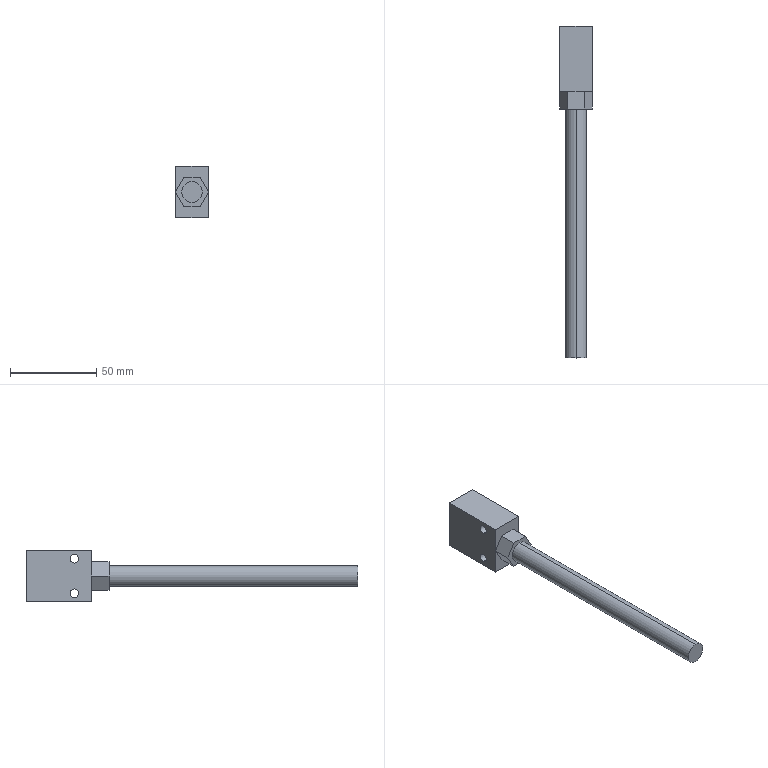Part | STEP file | Blowing port | 1 solid | 25 faces | box 19 x 192 x 30 mm | volume 38106 mm3 | plane 15 | cylinder 8 | cone 2 | commonest cylinder face diameters 5 x4 8.5 x2 12 x2
STEP:
#1=CARTESIAN_POINT('',(0.,-173.,6.));
#2=VERTEX_POINT('',#1);
#3=CARTESIAN_POINT('',(0.,-173.,-6.));
#4=VERTEX_POINT('',#3);
#5=CARTESIAN_POINT('',(0.,-173.,0.));
#6=DIRECTION('',(0.,1.,0.));
#7=DIRECTION('',(0.,0.,1.));
#8=AXIS2_PLACEMENT_3D('',#5,#6,#7);
#9=CIRCLE('',#8,6.);
#10=EDGE_CURVE('',#2,#4,#9,.T.);
#11=ORIENTED_EDGE('',*,*,#10,.T.);
#12=CARTESIAN_POINT('',(0.,-29.,-6.));
#13=VERTEX_POINT('',#12);
#14=CARTESIAN_POINT('',(0.,-173.,-6.));
#15=DIRECTION('',(0.,1.,0.));
#16=VECTOR('',#15,1000.);
#17=LINE('',#14,#16);
#18=EDGE_CURVE('',#4,#13,#17,.T.);
#19=ORIENTED_EDGE('',*,*,#18,.T.);
#20=CARTESIAN_POINT('',(0.,-29.,6.));
#21=VERTEX_POINT('',#20);
#22=CARTESIAN_POINT('',(0.,-29.,0.));
#23=DIRECTION('',(0.,-1.,0.));
#24=DIRECTION('',(0.,0.,1.));
#25=AXIS2_PLACEMENT_3D('',#22,#23,#24);
#26=CIRCLE('',#25,6.);
#27=EDGE_CURVE('',#13,#21,#26,.T.);
#28=ORIENTED_EDGE('',*,*,#27,.T.);
#29=CARTESIAN_POINT('',(0.,-173.,6.));
#30=DIRECTION('',(0.,1.,0.));
#31=VECTOR('',#30,1000.);
#32=LINE('',#29,#31);
#33=EDGE_CURVE('',#2,#21,#32,.T.);
#34=ORIENTED_EDGE('',*,*,#33,.F.);
#35=EDGE_LOOP('',(#11,#19,#28,#34));
#36=FACE_OUTER_BOUND('',#35,.T.);
#37=CARTESIAN_POINT('',(0.,-173.,0.));
#38=DIRECTION('',(0.,1.,0.));
#39=DIRECTION('',(0.,0.,1.));
#40=AXIS2_PLACEMENT_3D('',#37,#38,#39);
#41=CYLINDRICAL_SURFACE('',#40,6.);
#42=ADVANCED_FACE('',(#36),#41,.T.);
#43=CARTESIAN_POINT('',(9.5,-9.,-7.5));
#44=VERTEX_POINT('',#43);
#45=CARTESIAN_POINT('',(9.5,-9.,-12.5));
#46=VERTEX_POINT('',#45);
#47=CARTESIAN_POINT('',(9.5,-9.,-10.));
#48=DIRECTION('',(1.,0.,0.));
#49=DIRECTION('',(0.,0.,1.));
#50=AXIS2_PLACEMENT_3D('',#47,#48,#49);
#51=CIRCLE('',#50,2.5);
#52=EDGE_CURVE('',#44,#46,#51,.T.);
#53=ORIENTED_EDGE('',*,*,#52,.T.);
#54=CARTESIAN_POINT('',(-9.5,-9.,-12.5));
#55=VERTEX_POINT('',#54);
#56=CARTESIAN_POINT('',(9.5,-9.,-12.5));
#57=DIRECTION('',(-1.,0.,0.));
#58=VECTOR('',#57,1000.);
#59=LINE('',#56,#58);
#60=EDGE_CURVE('',#46,#55,#59,.T.);
#61=ORIENTED_EDGE('',*,*,#60,.T.);
#62=CARTESIAN_POINT('',(-9.5,-9.,-7.5));
#63=VERTEX_POINT('',#62);
#64=CARTESIAN_POINT('',(-9.5,-9.,-10.));
#65=DIRECTION('',(1.,0.,0.));
#66=DIRECTION('',(0.,0.,1.));
#67=AXIS2_PLACEMENT_3D('',#64,#65,#66);
#68=CIRCLE('',#67,2.5);
#69=EDGE_CURVE('',#63,#55,#68,.T.);
#70=ORIENTED_EDGE('',*,*,#69,.F.);
#71=CARTESIAN_POINT('',(9.5,-9.,-7.5));
#72=DIRECTION('',(-1.,0.,0.));
#73=VECTOR('',#72,1000.);
#74=LINE('',#71,#73);
#75=EDGE_CURVE('',#44,#63,#74,.T.);
#76=ORIENTED_EDGE('',*,*,#75,.F.);
#77=EDGE_LOOP('',(#53,#61,#70,#76));
#78=FACE_OUTER_BOUND('',#77,.T.);
#79=CARTESIAN_POINT('',(9.5,-9.,-10.));
#80=DIRECTION('',(-1.,0.,0.));
#81=DIRECTION('',(0.,0.,1.));
#82=AXIS2_PLACEMENT_3D('',#79,#80,#81);
#83=CYLINDRICAL_SURFACE('',#82,2.5);
#84=ADVANCED_FACE('',(#78),#83,.F.);
#85=CARTESIAN_POINT('',(9.5,-9.,12.5));
#86=VERTEX_POINT('',#85);
#87=CARTESIAN_POINT('',(9.5,-9.,7.5));
#88=VERTEX_POINT('',#87);
#89=CARTESIAN_POINT('',(9.5,-9.,10.));
#90=DIRECTION('',(1.,0.,0.));
#91=DIRECTION('',(0.,0.,1.));
#92=AXIS2_PLACEMENT_3D('',#89,#90,#91);
#93=CIRCLE('',#92,2.5);
#94=EDGE_CURVE('',#86,#88,#93,.T.);
#95=ORIENTED_EDGE('',*,*,#94,.T.);
#96=CARTESIAN_POINT('',(-9.5,-9.,7.5));
#97=VERTEX_POINT('',#96);
#98=CARTESIAN_POINT('',(9.5,-9.,7.5));
#99=DIRECTION('',(-1.,0.,0.));
#100=VECTOR('',#99,1000.);
#101=LINE('',#98,#100);
#102=EDGE_CURVE('',#88,#97,#101,.T.);
#103=ORIENTED_EDGE('',*,*,#102,.T.);
#104=CARTESIAN_POINT('',(-9.5,-9.,12.5));
#105=VERTEX_POINT('',#104);
#106=CARTESIAN_POINT('',(-9.5,-9.,10.));
#107=DIRECTION('',(1.,0.,0.));
#108=DIRECTION('',(0.,0.,1.));
#109=AXIS2_PLACEMENT_3D('',#106,#107,#108);
#110=CIRCLE('',#109,2.5);
#111=EDGE_CURVE('',#105,#97,#110,.T.);
#112=ORIENTED_EDGE('',*,*,#111,.F.);
#113=CARTESIAN_POINT('',(9.5,-9.,12.5));
#114=DIRECTION('',(-1.,0.,0.));
#115=VECTOR('',#114,1000.);
#116=LINE('',#113,#115);
#117=EDGE_CURVE('',#86,#105,#116,.T.);
#118=ORIENTED_EDGE('',*,*,#117,.F.);
#119=EDGE_LOOP('',(#95,#103,#112,#118));
#120=FACE_OUTER_BOUND('',#119,.T.);
#121=CARTESIAN_POINT('',(9.5,-9.,10.));
#122=DIRECTION('',(-1.,0.,0.));
#123=DIRECTION('',(0.,0.,1.));
#124=AXIS2_PLACEMENT_3D('',#121,#122,#123);
#125=CYLINDRICAL_SURFACE('',#124,2.5);
#126=ADVANCED_FACE('',(#120),#125,.F.);
#127=CARTESIAN_POINT('',(4.25,12.609,9.5));
#128=VERTEX_POINT('',#127);
#129=CARTESIAN_POINT('',(-4.25,12.609,9.5));
#130=VERTEX_POINT('',#129);
#131=CARTESIAN_POINT('',(0.,12.609,9.5));
#132=DIRECTION('',(0.,0.,-1.));
#133=DIRECTION('',(-1.,0.,0.));
#134=AXIS2_PLACEMENT_3D('',#131,#132,#133);
#135=CIRCLE('',#134,4.25);
#136=EDGE_CURVE('',#128,#130,#135,.T.);
#137=ORIENTED_EDGE('',*,*,#136,.F.);
#138=CARTESIAN_POINT('',(4.25,12.609,-15.));
#139=VERTEX_POINT('',#138);
#140=CARTESIAN_POINT('',(4.25,12.609,-15.));
#141=DIRECTION('',(0.,0.,-1.));
#142=VECTOR('',#141,1000.);
#143=LINE('',#140,#142);
#144=EDGE_CURVE('',#128,#139,#143,.T.);
#145=ORIENTED_EDGE('',*,*,#144,.T.);
#146=CARTESIAN_POINT('',(-4.25,12.609,-15.));
#147=VERTEX_POINT('',#146);
#148=CARTESIAN_POINT('',(0.,12.609,-15.));
#149=DIRECTION('',(0.,0.,-1.));
#150=DIRECTION('',(-1.,0.,0.));
#151=AXIS2_PLACEMENT_3D('',#148,#149,#150);
#152=CIRCLE('',#151,4.25);
#153=EDGE_CURVE('',#139,#147,#152,.T.);
#154=ORIENTED_EDGE('',*,*,#153,.T.);
#155=CARTESIAN_POINT('',(-4.25,12.609,-15.));
#156=DIRECTION('',(0.,0.,-1.));
#157=VECTOR('',#156,1000.);
#158=LINE('',#155,#157);
#159=EDGE_CURVE('',#130,#147,#158,.T.);
#160=ORIENTED_EDGE('',*,*,#159,.F.);
#161=EDGE_LOOP('',(#137,#145,#154,#160));
#162=FACE_OUTER_BOUND('',#161,.T.);
#163=CARTESIAN_POINT('',(0.,12.609,-15.));
#164=DIRECTION('',(0.,0.,-1.));
#165=DIRECTION('',(-1.,0.,0.));
#166=AXIS2_PLACEMENT_3D('',#163,#164,#165);
#167=CYLINDRICAL_SURFACE('',#166,4.25);
#168=ADVANCED_FACE('',(#162),#167,.F.);
#169=CARTESIAN_POINT('',(0.,12.609,12.054));
#170=VERTEX_POINT('',#169);
#171=CARTESIAN_POINT('',(-4.25,12.609,9.5));
#172=DIRECTION('',(-0.8572,0.,-0.515));
#173=VECTOR('',#172,1000.);
#174=LINE('',#171,#173);
#175=EDGE_CURVE('',#170,#130,#174,.T.);
#176=ORIENTED_EDGE('',*,*,#175,.F.);
#177=CARTESIAN_POINT('',(4.25,12.609,9.5));
#178=DIRECTION('',(0.8572,0.,-0.515));
#179=VECTOR('',#178,1000.);
#180=LINE('',#177,#179);
#181=EDGE_CURVE('',#170,#128,#180,.T.);
#182=ORIENTED_EDGE('',*,*,#181,.T.);
#183=ORIENTED_EDGE('',*,*,#136,.T.);
#184=EDGE_LOOP('',(#176,#182,#183));
#185=FACE_OUTER_BOUND('',#184,.T.);
#186=CARTESIAN_POINT('',(0.,12.609,9.5));
#187=DIRECTION('',(0.,0.,-1.));
#188=DIRECTION('',(-1.,0.,0.));
#189=AXIS2_PLACEMENT_3D('',#186,#187,#188);
#190=CONICAL_SURFACE('',#189,4.25,1.03);
#191=ADVANCED_FACE('',(#185),#190,.F.);
#192=ORIENTED_EDGE('',*,*,#18,.F.);
#193=CARTESIAN_POINT('',(0.,-173.,0.));
#194=DIRECTION('',(0.,1.,0.));
#195=DIRECTION('',(0.,0.,1.));
#196=AXIS2_PLACEMENT_3D('',#193,#194,#195);
#197=CIRCLE('',#196,6.);
#198=EDGE_CURVE('',#4,#2,#197,.T.);
#199=ORIENTED_EDGE('',*,*,#198,.T.);
#200=ORIENTED_EDGE('',*,*,#33,.T.);
#201=CARTESIAN_POINT('',(0.,-29.,0.));
#202=DIRECTION('',(0.,-1.,0.));
#203=DIRECTION('',(0.,0.,1.));
#204=AXIS2_PLACEMENT_3D('',#201,#202,#203);
#205=CIRCLE('',#204,6.);
#206=EDGE_CURVE('',#21,#13,#205,.T.);
#207=ORIENTED_EDGE('',*,*,#206,.T.);
#208=EDGE_LOOP('',(#192,#199,#200,#207));
#209=FACE_OUTER_BOUND('',#208,.T.);
#210=CARTESIAN_POINT('',(0.,-173.,0.));
#211=DIRECTION('',(0.,1.,0.));
#212=DIRECTION('',(0.,0.,1.));
#213=AXIS2_PLACEMENT_3D('',#210,#211,#212);
#214=CYLINDRICAL_SURFACE('',#213,6.);
#215=ADVANCED_FACE('',(#209),#214,.T.);
#216=CARTESIAN_POINT('',(-9.5,-29.,0.));
#217=VERTEX_POINT('',#216);
#218=CARTESIAN_POINT('',(-4.75,-29.,-8.227));
#219=VERTEX_POINT('',#218);
#220=CARTESIAN_POINT('',(-9.5,-29.,0.));
#221=DIRECTION('',(0.5,0.,-0.866));
#222=VECTOR('',#221,1000.);
#223=LINE('',#220,#222);
#224=EDGE_CURVE('',#217,#219,#223,.T.);
#225=ORIENTED_EDGE('',*,*,#224,.T.);
#226=CARTESIAN_POINT('',(4.75,-29.,-8.227));
#227=VERTEX_POINT('',#226);
#228=CARTESIAN_POINT('',(0.,-29.,-8.227));
#229=DIRECTION('',(1.,0.,0.));
#230=VECTOR('',#229,1000.);
#231=LINE('',#228,#230);
#232=EDGE_CURVE('',#219,#227,#231,.T.);
#233=ORIENTED_EDGE('',*,*,#232,.T.);
#234=CARTESIAN_POINT('',(9.5,-29.,0.));
#235=VERTEX_POINT('',#234);
#236=CARTESIAN_POINT('',(4.75,-29.,-8.227));
#237=DIRECTION('',(0.5,0.,0.866));
#238=VECTOR('',#237,1000.);
#239=LINE('',#236,#238);
#240=EDGE_CURVE('',#227,#235,#239,.T.);
#241=ORIENTED_EDGE('',*,*,#240,.T.);
#242=CARTESIAN_POINT('',(4.75,-29.,8.227));
#243=VERTEX_POINT('',#242);
#244=CARTESIAN_POINT('',(9.5,-29.,0.));
#245=DIRECTION('',(-0.5,0.,0.866));
#246=VECTOR('',#245,1000.);
#247=LINE('',#244,#246);
#248=EDGE_CURVE('',#235,#243,#247,.T.);
#249=ORIENTED_EDGE('',*,*,#248,.T.);
#250=CARTESIAN_POINT('',(-4.75,-29.,8.227));
#251=VERTEX_POINT('',#250);
#252=CARTESIAN_POINT('',(0.,-29.,8.227));
#253=DIRECTION('',(-1.,0.,0.));
#254=VECTOR('',#253,1000.);
#255=LINE('',#252,#254);
#256=EDGE_CURVE('',#243,#251,#255,.T.);
#257=ORIENTED_EDGE('',*,*,#256,.T.);
#258=CARTESIAN_POINT('',(-4.75,-29.,8.227));
#259=DIRECTION('',(-0.5,0.,-0.866));
#260=VECTOR('',#259,1000.);
#261=LINE('',#258,#260);
#262=EDGE_CURVE('',#251,#217,#261,.T.);
#263=ORIENTED_EDGE('',*,*,#262,.T.);
#264=EDGE_LOOP('',(#225,#233,#241,#249,#257,#263));
#265=FACE_OUTER_BOUND('',#264,.T.);
#266=ORIENTED_EDGE('',*,*,#206,.F.);
#267=ORIENTED_EDGE('',*,*,#27,.F.);
#268=EDGE_LOOP('',(#266,#267));
#269=FACE_BOUND('',#268,.T.);
#270=CARTESIAN_POINT('',(0.,-29.,0.));
#271=DIRECTION('',(0.,-1.,0.));
#272=DIRECTION('',(0.,0.,-1.));
#273=AXIS2_PLACEMENT_3D('',#270,#271,#272);
#274=PLANE('',#273);
#275=ADVANCED_FACE('',(#265,#269),#274,.T.);
#276=ORIENTED_EDGE('',*,*,#10,.F.);
#277=ORIENTED_EDGE('',*,*,#198,.F.);
#278=EDGE_LOOP('',(#276,#277));
#279=FACE_OUTER_BOUND('',#278,.T.);
#280=CARTESIAN_POINT('',(0.,-173.,0.));
#281=DIRECTION('',(0.,-1.,0.));
#282=DIRECTION('',(0.,0.,-1.));
#283=AXIS2_PLACEMENT_3D('',#280,#281,#282);
#284=PLANE('',#283);
#285=ADVANCED_FACE('',(#279),#284,.T.);
#286=CARTESIAN_POINT('',(4.75,-19.,-8.227));
#287=VERTEX_POINT('',#286);
#288=CARTESIAN_POINT('',(4.75,-29.,-8.227));
#289=DIRECTION('',(0.,1.,0.));
#290=VECTOR('',#289,1000.);
#291=LINE('',#288,#290);
#292=EDGE_CURVE('',#227,#287,#291,.T.);
#293=ORIENTED_EDGE('',*,*,#292,.F.);
#294=ORIENTED_EDGE('',*,*,#232,.F.);
#295=CARTESIAN_POINT('',(-4.75,-19.,-8.227));
#296=VERTEX_POINT('',#295);
#297=CARTESIAN_POINT('',(-4.75,-29.,-8.227));
#298=DIRECTION('',(0.,-1.,0.));
#299=VECTOR('',#298,1000.);
#300=LINE('',#297,#299);
#301=EDGE_CURVE('',#296,#219,#300,.T.);
#302=ORIENTED_EDGE('',*,*,#301,.F.);
#303=CARTESIAN_POINT('',(-4.75,-19.,-8.227));
#304=DIRECTION('',(-1.,0.,0.));
#305=VECTOR('',#304,1000.);
#306=LINE('',#303,#305);
#307=EDGE_CURVE('',#287,#296,#306,.T.);
#308=ORIENTED_EDGE('',*,*,#307,.F.);
#309=EDGE_LOOP('',(#293,#294,#302,#308));
#310=FACE_OUTER_BOUND('',#309,.T.);
#311=CARTESIAN_POINT('',(-4.75,-29.,-8.227));
#312=DIRECTION('',(0.,0.,1.));
#313=DIRECTION('',(1.,0.,0.));
#314=AXIS2_PLACEMENT_3D('',#311,#312,#313);
#315=PLANE('',#314);
#316=ADVANCED_FACE('',(#310),#315,.F.);
#317=ORIENTED_EDGE('',*,*,#301,.T.);
#318=ORIENTED_EDGE('',*,*,#224,.F.);
#319=CARTESIAN_POINT('',(-9.5,-19.,0.));
#320=VERTEX_POINT('',#319);
#321=CARTESIAN_POINT('',(-9.5,-29.,0.));
#322=DIRECTION('',(0.,-1.,0.));
#323=VECTOR('',#322,1000.);
#324=LINE('',#321,#323);
#325=EDGE_CURVE('',#320,#217,#324,.T.);
#326=ORIENTED_EDGE('',*,*,#325,.F.);
#327=CARTESIAN_POINT('',(-9.5,-19.,0.));
#328=DIRECTION('',(-0.5,0.,0.866));
#329=VECTOR('',#328,1000.);
#330=LINE('',#327,#329);
#331=EDGE_CURVE('',#296,#320,#330,.T.);
#332=ORIENTED_EDGE('',*,*,#331,.F.);
#333=EDGE_LOOP('',(#317,#318,#326,#332));
#334=FACE_OUTER_BOUND('',#333,.T.);
#335=CARTESIAN_POINT('',(-9.5,-29.,0.));
#336=DIRECTION('',(0.866,0.,0.5));
#337=DIRECTION('',(0.5,0.,-0.866));
#338=AXIS2_PLACEMENT_3D('',#335,#336,#337);
#339=PLANE('',#338);
#340=ADVANCED_FACE('',(#334),#339,.F.);
#341=ORIENTED_EDGE('',*,*,#325,.T.);
#342=ORIENTED_EDGE('',*,*,#262,.F.);
#343=CARTESIAN_POINT('',(-4.75,-19.,8.227));
#344=VERTEX_POINT('',#343);
#345=CARTESIAN_POINT('',(-4.75,-29.,8.227));
#346=DIRECTION('',(0.,-1.,0.));
#347=VECTOR('',#346,1000.);
#348=LINE('',#345,#347);
#349=EDGE_CURVE('',#344,#251,#348,.T.);
#350=ORIENTED_EDGE('',*,*,#349,.F.);
#351=CARTESIAN_POINT('',(-4.75,-19.,8.227));
#352=DIRECTION('',(0.5,0.,0.866));
#353=VECTOR('',#352,1000.);
#354=LINE('',#351,#353);
#355=EDGE_CURVE('',#320,#344,#354,.T.);
#356=ORIENTED_EDGE('',*,*,#355,.F.);
#357=EDGE_LOOP('',(#341,#342,#350,#356));
#358=FACE_OUTER_BOUND('',#357,.T.);
#359=CARTESIAN_POINT('',(-4.75,-29.,8.227));
#360=DIRECTION('',(0.866,0.,-0.5));
#361=DIRECTION('',(-0.5,0.,-0.866));
#362=AXIS2_PLACEMENT_3D('',#359,#360,#361);
#363=PLANE('',#362);
#364=ADVANCED_FACE('',(#358),#363,.F.);
#365=ORIENTED_EDGE('',*,*,#349,.T.);
#366=ORIENTED_EDGE('',*,*,#256,.F.);
#367=CARTESIAN_POINT('',(4.75,-19.,8.227));
#368=VERTEX_POINT('',#367);
#369=CARTESIAN_POINT('',(4.75,-29.,8.227));
#370=DIRECTION('',(0.,-1.,0.));
#371=VECTOR('',#370,1000.);
#372=LINE('',#369,#371);
#373=EDGE_CURVE('',#368,#243,#372,.T.);
#374=ORIENTED_EDGE('',*,*,#373,.F.);
#375=CARTESIAN_POINT('',(4.75,-19.,8.227));
#376=DIRECTION('',(1.,0.,0.));
#377=VECTOR('',#376,1000.);
#378=LINE('',#375,#377);
#379=EDGE_CURVE('',#344,#368,#378,.T.);
#380=ORIENTED_EDGE('',*,*,#379,.F.);
#381=EDGE_LOOP('',(#365,#366,#374,#380));
#382=FACE_OUTER_BOUND('',#381,.T.);
#383=CARTESIAN_POINT('',(4.75,-29.,8.227));
#384=DIRECTION('',(0.,0.,-1.));
#385=DIRECTION('',(-1.,0.,0.));
#386=AXIS2_PLACEMENT_3D('',#383,#384,#385);
#387=PLANE('',#386);
#388=ADVANCED_FACE('',(#382),#387,.F.);
#389=ORIENTED_EDGE('',*,*,#373,.T.);
#390=ORIENTED_EDGE('',*,*,#248,.F.);
#391=CARTESIAN_POINT('',(9.5,-19.,0.));
#392=VERTEX_POINT('',#391);
#393=CARTESIAN_POINT('',(9.5,-29.,0.));
#394=DIRECTION('',(0.,-1.,0.));
#395=VECTOR('',#394,1000.);
#396=LINE('',#393,#395);
#397=EDGE_CURVE('',#392,#235,#396,.T.);
#398=ORIENTED_EDGE('',*,*,#397,.F.);
#399=CARTESIAN_POINT('',(9.5,-19.,0.));
#400=DIRECTION('',(0.5,0.,-0.866));
#401=VECTOR('',#400,1000.);
#402=LINE('',#399,#401);
#403=EDGE_CURVE('',#368,#392,#402,.T.);
#404=ORIENTED_EDGE('',*,*,#403,.F.);
#405=EDGE_LOOP('',(#389,#390,#398,#404));
#406=FACE_OUTER_BOUND('',#405,.T.);
#407=CARTESIAN_POINT('',(9.5,-29.,0.));
#408=DIRECTION('',(-0.866,0.,-0.5));
#409=DIRECTION('',(-0.5,0.,0.866));
#410=AXIS2_PLACEMENT_3D('',#407,#408,#409);
#411=PLANE('',#410);
#412=ADVANCED_FACE('',(#406),#411,.F.);
#413=ORIENTED_EDGE('',*,*,#397,.T.);
#414=ORIENTED_EDGE('',*,*,#240,.F.);
#415=ORIENTED_EDGE('',*,*,#292,.T.);
#416=CARTESIAN_POINT('',(4.75,-19.,-8.227));
#417=DIRECTION('',(-0.5,0.,-0.866));
#418=VECTOR('',#417,1000.);
#419=LINE('',#416,#418);
#420=EDGE_CURVE('',#392,#287,#419,.T.);
#421=ORIENTED_EDGE('',*,*,#420,.F.);
#422=EDGE_LOOP('',(#413,#414,#415,#421));
#423=FACE_OUTER_BOUND('',#422,.T.);
#424=CARTESIAN_POINT('',(4.75,-29.,-8.227));
#425=DIRECTION('',(-0.866,0.,0.5));
#426=DIRECTION('',(0.5,0.,0.866));
#427=AXIS2_PLACEMENT_3D('',#424,#425,#426);
#428=PLANE('',#427);
#429=ADVANCED_FACE('',(#423),#428,.F.);
#430=ORIENTED_EDGE('',*,*,#307,.T.);
#431=ORIENTED_EDGE('',*,*,#331,.T.);
#432=CARTESIAN_POINT('',(-9.5,-19.,-15.));
#433=VERTEX_POINT('',#432);
#434=CARTESIAN_POINT('',(-9.5,-19.,15.));
#435=DIRECTION('',(0.,0.,1.));
#436=VECTOR('',#435,1000.);
#437=LINE('',#434,#436);
#438=EDGE_CURVE('',#433,#320,#437,.T.);
#439=ORIENTED_EDGE('',*,*,#438,.F.);
#440=CARTESIAN_POINT('',(9.5,-19.,-15.));
#441=VERTEX_POINT('',#440);
#442=CARTESIAN_POINT('',(9.5,-19.,-15.));
#443=DIRECTION('',(-1.,0.,0.));
#444=VECTOR('',#443,1000.);
#445=LINE('',#442,#444);
#446=EDGE_CURVE('',#441,#433,#445,.T.);
#447=ORIENTED_EDGE('',*,*,#446,.F.);
#448=CARTESIAN_POINT('',(9.5,-19.,15.));
#449=DIRECTION('',(0.,0.,-1.));
#450=VECTOR('',#449,1000.);
#451=LINE('',#448,#450);
#452=EDGE_CURVE('',#392,#441,#451,.T.);
#453=ORIENTED_EDGE('',*,*,#452,.F.);
#454=ORIENTED_EDGE('',*,*,#420,.T.);
#455=EDGE_LOOP('',(#430,#431,#439,#447,#453,#454));
#456=FACE_OUTER_BOUND('',#455,.T.);
#457=CARTESIAN_POINT('',(9.5,-19.,15.));
#458=DIRECTION('',(0.,1.,0.));
#459=DIRECTION('',(0.,0.,1.));
#460=AXIS2_PLACEMENT_3D('',#457,#458,#459);
#461=PLANE('',#460);
#462=ADVANCED_FACE('',(#456),#461,.F.);
#463=ORIENTED_EDGE('',*,*,#379,.T.);
#464=ORIENTED_EDGE('',*,*,#403,.T.);
#465=CARTESIAN_POINT('',(9.5,-19.,15.));
#466=VERTEX_POINT('',#465);
#467=CARTESIAN_POINT('',(9.5,-19.,15.));
#468=DIRECTION('',(0.,0.,-1.));
#469=VECTOR('',#468,1000.);
#470=LINE('',#467,#469);
#471=EDGE_CURVE('',#466,#392,#470,.T.);
#472=ORIENTED_EDGE('',*,*,#471,.F.);
#473=CARTESIAN_POINT('',(-9.5,-19.,15.));
#474=VERTEX_POINT('',#473);
#475=CARTESIAN_POINT('',(9.5,-19.,15.));
#476=DIRECTION('',(1.,0.,0.));
#477=VECTOR('',#476,1000.);
#478=LINE('',#475,#477);
#479=EDGE_CURVE('',#474,#466,#478,.T.);
#480=ORIENTED_EDGE('',*,*,#479,.F.);
#481=CARTESIAN_POINT('',(-9.5,-19.,15.));
#482=DIRECTION('',(0.,0.,1.));
#483=VECTOR('',#482,1000.);
#484=LINE('',#481,#483);
#485=EDGE_CURVE('',#320,#474,#484,.T.);
#486=ORIENTED_EDGE('',*,*,#485,.F.);
#487=ORIENTED_EDGE('',*,*,#355,.T.);
#488=EDGE_LOOP('',(#463,#464,#472,#480,#486,#487));
#489=FACE_OUTER_BOUND('',#488,.T.);
#490=CARTESIAN_POINT('',(9.5,-19.,15.));
#491=DIRECTION('',(0.,1.,0.));
#492=DIRECTION('',(0.,0.,1.));
#493=AXIS2_PLACEMENT_3D('',#490,#491,#492);
#494=PLANE('',#493);
#495=ADVANCED_FACE('',(#489),#494,.F.);
#496=ORIENTED_EDGE('',*,*,#69,.T.);
#497=CARTESIAN_POINT('',(-9.5,-9.,-10.));
#498=DIRECTION('',(1.,0.,0.));
#499=DIRECTION('',(0.,0.,1.));
#500=AXIS2_PLACEMENT_3D('',#497,#498,#499);
#501=CIRCLE('',#500,2.5);
#502=EDGE_CURVE('',#55,#63,#501,.T.);
#503=ORIENTED_EDGE('',*,*,#502,.T.);
#504=EDGE_LOOP('',(#496,#503));
#505=FACE_BOUND('',#504,.T.);
#506=ORIENTED_EDGE('',*,*,#438,.T.);
#507=ORIENTED_EDGE('',*,*,#485,.T.);
#508=CARTESIAN_POINT('',(-9.5,19.,15.));
#509=VERTEX_POINT('',#508);
#510=CARTESIAN_POINT('',(-9.5,0.,15.));
#511=DIRECTION('',(0.,1.,0.));
#512=VECTOR('',#511,1000.);
#513=LINE('',#510,#512);
#514=EDGE_CURVE('',#474,#509,#513,.T.);
#515=ORIENTED_EDGE('',*,*,#514,.T.);
#516=CARTESIAN_POINT('',(-9.5,19.,-15.));
#517=VERTEX_POINT('',#516);
#518=CARTESIAN_POINT('',(-9.5,19.,0.));
#519=DIRECTION('',(0.,0.,-1.));
#520=VECTOR('',#519,1000.);
#521=LINE('',#518,#520);
#522=EDGE_CURVE('',#509,#517,#521,.T.);
#523=ORIENTED_EDGE('',*,*,#522,.T.);
#524=CARTESIAN_POINT('',(-9.5,0.,-15.));
#525=DIRECTION('',(0.,-1.,0.));
#526=VECTOR('',#525,1000.);
#527=LINE('',#524,#526);
#528=EDGE_CURVE('',#517,#433,#527,.T.);
#529=ORIENTED_EDGE('',*,*,#528,.T.);
#530=EDGE_LOOP('',(#506,#507,#515,#523,#529));
#531=FACE_OUTER_BOUND('',#530,.T.);
#532=ORIENTED_EDGE('',*,*,#111,.T.);
#533=CARTESIAN_POINT('',(-9.5,-9.,10.));
#534=DIRECTION('',(1.,0.,0.));
#535=DIRECTION('',(0.,0.,1.));
#536=AXIS2_PLACEMENT_3D('',#533,#534,#535);
#537=CIRCLE('',#536,2.5);
#538=EDGE_CURVE('',#97,#105,#537,.T.);
#539=ORIENTED_EDGE('',*,*,#538,.T.);
#540=EDGE_LOOP('',(#532,#539));
#541=FACE_BOUND('',#540,.T.);
#542=CARTESIAN_POINT('',(-9.5,0.,0.));
#543=DIRECTION('',(-1.,0.,0.));
#544=DIRECTION('',(0.,0.,1.));
#545=AXIS2_PLACEMENT_3D('',#542,#543,#544);
#546=PLANE('',#545);
#547=ADVANCED_FACE('',(#505,#531,#541),#546,.T.);
#548=CARTESIAN_POINT('',(9.5,19.,-15.));
#549=VERTEX_POINT('',#548);
#550=CARTESIAN_POINT('',(9.5,19.,-15.));
#551=DIRECTION('',(-1.,0.,0.));
#552=VECTOR('',#551,1000.);
#553=LINE('',#550,#552);
#554=EDGE_CURVE('',#549,#517,#553,.T.);
#555=ORIENTED_EDGE('',*,*,#554,.F.);
#556=CARTESIAN_POINT('',(9.5,-19.,-15.));
#557=DIRECTION('',(0.,1.,0.));
#558=VECTOR('',#557,1000.);
#559=LINE('',#556,#558);
#560=EDGE_CURVE('',#441,#549,#559,.T.);
#561=ORIENTED_EDGE('',*,*,#560,.F.);
#562=ORIENTED_EDGE('',*,*,#446,.T.);
#563=ORIENTED_EDGE('',*,*,#528,.F.);
#564=EDGE_LOOP('',(#555,#561,#562,#563));
#565=FACE_OUTER_BOUND('',#564,.T.);
#566=CARTESIAN_POINT('',(0.,12.609,-15.));
#567=DIRECTION('',(0.,0.,-1.));
#568=DIRECTION('',(-1.,0.,0.));
#569=AXIS2_PLACEMENT_3D('',#566,#567,#568);
#570=CIRCLE('',#569,4.25);
#571=EDGE_CURVE('',#147,#139,#570,.T.);
#572=ORIENTED_EDGE('',*,*,#571,.F.);
#573=ORIENTED_EDGE('',*,*,#153,.F.);
#574=EDGE_LOOP('',(#572,#573));
#575=FACE_BOUND('',#574,.T.);
#576=CARTESIAN_POINT('',(9.5,-19.,-15.));
#577=DIRECTION('',(0.,0.,1.));
#578=DIRECTION('',(1.,0.,0.));
#579=AXIS2_PLACEMENT_3D('',#576,#577,#578);
#580=PLANE('',#579);
#581=ADVANCED_FACE('',(#565,#575),#580,.F.);
#582=ORIENTED_EDGE('',*,*,#52,.F.);
#583=CARTESIAN_POINT('',(9.5,-9.,-10.));
#584=DIRECTION('',(1.,0.,0.));
#585=DIRECTION('',(0.,0.,1.));
#586=AXIS2_PLACEMENT_3D('',#583,#584,#585);
#587=CIRCLE('',#586,2.5);
#588=EDGE_CURVE('',#46,#44,#587,.T.);
#589=ORIENTED_EDGE('',*,*,#588,.F.);
#590=EDGE_LOOP('',(#582,#589));
#591=FACE_BOUND('',#590,.T.);
#592=ORIENTED_EDGE('',*,*,#94,.F.);
#593=CARTESIAN_POINT('',(9.5,-9.,10.));
#594=DIRECTION('',(1.,0.,0.));
#595=DIRECTION('',(0.,0.,1.));
#596=AXIS2_PLACEMENT_3D('',#593,#594,#595);
#597=CIRCLE('',#596,2.5);
#598=EDGE_CURVE('',#88,#86,#597,.T.);
#599=ORIENTED_EDGE('',*,*,#598,.F.);
#600=EDGE_LOOP('',(#592,#599));
#601=FACE_BOUND('',#600,.T.);
#602=ORIENTED_EDGE('',*,*,#471,.T.);
#603=ORIENTED_EDGE('',*,*,#452,.T.);
#604=ORIENTED_EDGE('',*,*,#560,.T.);
#605=CARTESIAN_POINT('',(9.5,19.,15.));
#606=VERTEX_POINT('',#605);
#607=CARTESIAN_POINT('',(9.5,19.,0.));
#608=DIRECTION('',(0.,0.,-1.));
#609=VECTOR('',#608,1000.);
#610=LINE('',#607,#609);
#611=EDGE_CURVE('',#606,#549,#610,.T.);
#612=ORIENTED_EDGE('',*,*,#611,.F.);
#613=CARTESIAN_POINT('',(9.5,0.,15.));
#614=DIRECTION('',(0.,1.,0.));
#615=VECTOR('',#614,1000.);
#616=LINE('',#613,#615);
#617=EDGE_CURVE('',#466,#606,#616,.T.);
#618=ORIENTED_EDGE('',*,*,#617,.F.);
#619=EDGE_LOOP('',(#602,#603,#604,#612,#618));
#620=FACE_OUTER_BOUND('',#619,.T.);
#621=CARTESIAN_POINT('',(9.5,0.,0.));
#622=DIRECTION('',(-1.,0.,0.));
#623=DIRECTION('',(0.,0.,1.));
#624=AXIS2_PLACEMENT_3D('',#621,#622,#623);
#625=PLANE('',#624);
#626=ADVANCED_FACE('',(#591,#601,#620),#625,.F.);
#627=ORIENTED_EDGE('',*,*,#617,.T.);
#628=CARTESIAN_POINT('',(9.5,19.,15.));
#629=DIRECTION('',(-1.,0.,0.));
#630=VECTOR('',#629,1000.);
#631=LINE('',#628,#630);
#632=EDGE_CURVE('',#606,#509,#631,.T.);
#633=ORIENTED_EDGE('',*,*,#632,.T.);
#634=ORIENTED_EDGE('',*,*,#514,.F.);
#635=ORIENTED_EDGE('',*,*,#479,.T.);
#636=EDGE_LOOP('',(#627,#633,#634,#635));
#637=FACE_OUTER_BOUND('',#636,.T.);
#638=CARTESIAN_POINT('',(9.5,-19.,15.));
#639=DIRECTION('',(0.,0.,1.));
#640=DIRECTION('',(1.,0.,0.));
#641=AXIS2_PLACEMENT_3D('',#638,#639,#640);
#642=PLANE('',#641);
#643=ADVANCED_FACE('',(#637),#642,.T.);
#644=ORIENTED_EDGE('',*,*,#60,.F.);
#645=ORIENTED_EDGE('',*,*,#588,.T.);
#646=ORIENTED_EDGE('',*,*,#75,.T.);
#647=ORIENTED_EDGE('',*,*,#502,.F.);
#648=EDGE_LOOP('',(#644,#645,#646,#647));
#649=FACE_OUTER_BOUND('',#648,.T.);
#650=CARTESIAN_POINT('',(9.5,-9.,-10.));
#651=DIRECTION('',(-1.,0.,0.));
#652=DIRECTION('',(0.,0.,1.));
#653=AXIS2_PLACEMENT_3D('',#650,#651,#652);
#654=CYLINDRICAL_SURFACE('',#653,2.5);
#655=ADVANCED_FACE('',(#649),#654,.F.);
#656=ORIENTED_EDGE('',*,*,#611,.T.);
#657=ORIENTED_EDGE('',*,*,#554,.T.);
#658=ORIENTED_EDGE('',*,*,#522,.F.);
#659=ORIENTED_EDGE('',*,*,#632,.F.);
#660=EDGE_LOOP('',(#656,#657,#658,#659));
#661=FACE_OUTER_BOUND('',#660,.T.);
#662=CARTESIAN_POINT('',(9.5,19.,15.));
#663=DIRECTION('',(0.,1.,0.));
#664=DIRECTION('',(0.,0.,1.));
#665=AXIS2_PLACEMENT_3D('',#662,#663,#664);
#666=PLANE('',#665);
#667=ADVANCED_FACE('',(#661),#666,.T.);
#668=ORIENTED_EDGE('',*,*,#102,.F.);
#669=ORIENTED_EDGE('',*,*,#598,.T.);
#670=ORIENTED_EDGE('',*,*,#117,.T.);
#671=ORIENTED_EDGE('',*,*,#538,.F.);
#672=EDGE_LOOP('',(#668,#669,#670,#671));
#673=FACE_OUTER_BOUND('',#672,.T.);
#674=CARTESIAN_POINT('',(9.5,-9.,10.));
#675=DIRECTION('',(-1.,0.,0.));
#676=DIRECTION('',(0.,0.,1.));
#677=AXIS2_PLACEMENT_3D('',#674,#675,#676);
#678=CYLINDRICAL_SURFACE('',#677,2.5);
#679=ADVANCED_FACE('',(#673),#678,.F.);
#680=ORIENTED_EDGE('',*,*,#144,.F.);
#681=CARTESIAN_POINT('',(0.,12.609,9.5));
#682=DIRECTION('',(0.,0.,-1.));
#683=DIRECTION('',(-1.,0.,0.));
#684=AXIS2_PLACEMENT_3D('',#681,#682,#683);
#685=CIRCLE('',#684,4.25);
#686=EDGE_CURVE('',#130,#128,#685,.T.);
#687=ORIENTED_EDGE('',*,*,#686,.F.);
#688=ORIENTED_EDGE('',*,*,#159,.T.);
#689=ORIENTED_EDGE('',*,*,#571,.T.);
#690=EDGE_LOOP('',(#680,#687,#688,#689));
#691=FACE_OUTER_BOUND('',#690,.T.);
#692=CARTESIAN_POINT('',(0.,12.609,-15.));
#693=DIRECTION('',(0.,0.,-1.));
#694=DIRECTION('',(-1.,0.,0.));
#695=AXIS2_PLACEMENT_3D('',#692,#693,#694);
#696=CYLINDRICAL_SURFACE('',#695,4.25);
#697=ADVANCED_FACE('',(#691),#696,.F.);
#698=ORIENTED_EDGE('',*,*,#181,.F.);
#699=ORIENTED_EDGE('',*,*,#175,.T.);
#700=ORIENTED_EDGE('',*,*,#686,.T.);
#701=EDGE_LOOP('',(#698,#699,#700));
#702=FACE_OUTER_BOUND('',#701,.T.);
#703=CARTESIAN_POINT('',(0.,12.609,9.5));
#704=DIRECTION('',(0.,0.,-1.));
#705=DIRECTION('',(-1.,0.,0.));
#706=AXIS2_PLACEMENT_3D('',#703,#704,#705);
#707=CONICAL_SURFACE('',#706,4.25,1.03);
#708=ADVANCED_FACE('',(#702),#707,.F.);
#709=CLOSED_SHELL('',(#42,#84,#126,#168,#191,#215,#275,#285,#316,#340,#364,#388,#412,#429,#462,#495,#547,#581,#626,#643,#655,#667,#679,#697,#708));
#710=MANIFOLD_SOLID_BREP('',#709);
#711=CARTESIAN_POINT('',(0.,0.,0.));
#712=DIRECTION('',(0.,0.,1.));
#713=DIRECTION('',(1.,0.,0.));
#714=AXIS2_PLACEMENT_3D('',#711,#712,#713);
#715=(LENGTH_UNIT()NAMED_UNIT(*)SI_UNIT(.MILLI.,.METRE.));
#716=UNCERTAINTY_MEASURE_WITH_UNIT(LENGTH_MEASURE(0.00001),#715,'','');
#717=(NAMED_UNIT(*)PLANE_ANGLE_UNIT()SI_UNIT($,.RADIAN.));
#718=(NAMED_UNIT(*)SI_UNIT($,.STERADIAN.)SOLID_ANGLE_UNIT());
#719=(GEOMETRIC_REPRESENTATION_CONTEXT(3)GLOBAL_UNCERTAINTY_ASSIGNED_CONTEXT((#716))GLOBAL_UNIT_ASSIGNED_CONTEXT((#715,#717,#718))REPRESENTATION_CONTEXT('',''));
#720=ADVANCED_BREP_SHAPE_REPRESENTATION('',(#710,#714),#719);